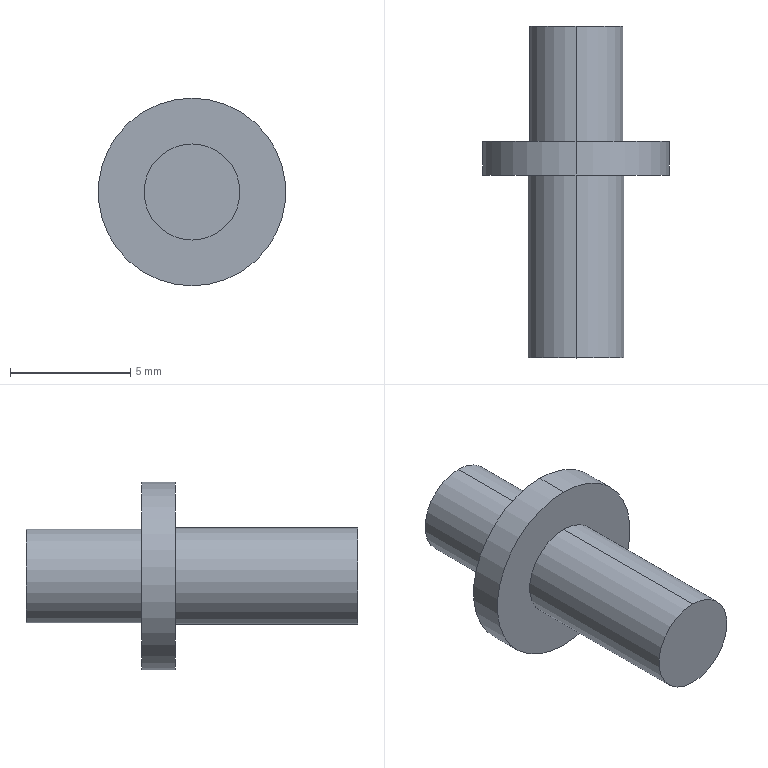Part | STEP file | Hinge lower door shaft 001 | 1 solid | 10 faces | box 7.8 x 13.8 x 7.8 mm | volume 219.742 mm3 | cylinder 6 | plane 4 | commonest cylinder face diameters 3.9 x2 4 x2 7.8 x2
STEP:
#1=CARTESIAN_POINT('',(0.,0.,0.));
#2=DIRECTION('',(0.,0.,1.));
#3=DIRECTION('',(1.,0.,0.));
#4=AXIS2_PLACEMENT_3D('',#1,#2,#3);
#5=CARTESIAN_POINT('',(0.,13.8,1.95));
#6=VERTEX_POINT('',#5);
#7=CARTESIAN_POINT('',(0.,13.8,-1.95));
#8=VERTEX_POINT('',#7);
#9=CARTESIAN_POINT('',(0.,13.8,0.));
#10=DIRECTION('',(0.,1.,0.));
#11=DIRECTION('',(0.,0.,1.));
#12=AXIS2_PLACEMENT_3D('',#9,#10,#11);
#13=CIRCLE('',#12,1.95);
#14=CARTESIAN_POINT('',(0.,13.8,0.));
#15=DIRECTION('',(0.,-1.,0.));
#16=DIRECTION('',(0.,0.,-1.));
#17=AXIS2_PLACEMENT_3D('',#14,#15,#16);
#18=CYLINDRICAL_SURFACE('',#17,1.95);
#19=CARTESIAN_POINT('',(3.142,0.));
#20=DIRECTION('',(-1.,0.));
#21=VECTOR('',#20,1.);
#22=LINE('',#19,#21);
#23=(GEOMETRIC_REPRESENTATION_CONTEXT(2)PARAMETRIC_REPRESENTATION_CONTEXT()REPRESENTATION_CONTEXT('',''));
#24=DEFINITIONAL_REPRESENTATION('',(#22),#23);
#25=PCURVE('',#18,#24);
#26=CARTESIAN_POINT('',(0.,13.8,0.));
#27=DIRECTION('',(0.,1.,0.));
#28=DIRECTION('',(1.,0.,0.));
#29=AXIS2_PLACEMENT_3D('',#26,#27,#28);
#30=PLANE('',#29);
#31=CARTESIAN_POINT('',(0.,0.));
#32=DIRECTION('',(0.,-1.));
#33=AXIS2_PLACEMENT_2D('',#31,#32);
#34=CIRCLE('',#33,1.95);
#35=(GEOMETRIC_REPRESENTATION_CONTEXT(2)PARAMETRIC_REPRESENTATION_CONTEXT()REPRESENTATION_CONTEXT('',''));
#36=DEFINITIONAL_REPRESENTATION('',(#34),#35);
#37=PCURVE('',#30,#36);
#38=SURFACE_CURVE('',#13,(#25,#37),.PCURVE_S1.);
#39=EDGE_CURVE('',#6,#8,#38,.T.);
#40=ORIENTED_EDGE('',*,*,#39,.F.);
#41=CARTESIAN_POINT('',(0.,9.,1.95));
#42=VERTEX_POINT('',#41);
#43=CARTESIAN_POINT('',(0.,13.8,1.95));
#44=DIRECTION('',(0.,-1.,0.));
#45=VECTOR('',#44,1.);
#46=LINE('',#43,#45);
#47=CARTESIAN_POINT('',(3.142,0.));
#48=DIRECTION('',(0.,1.));
#49=VECTOR('',#48,1.);
#50=LINE('',#47,#49);
#51=(GEOMETRIC_REPRESENTATION_CONTEXT(2)PARAMETRIC_REPRESENTATION_CONTEXT()REPRESENTATION_CONTEXT('',''));
#52=DEFINITIONAL_REPRESENTATION('',(#50),#51);
#53=PCURVE('',#18,#52);
#54=CARTESIAN_POINT('',(0.,13.8,0.));
#55=DIRECTION('',(0.,-1.,0.));
#56=DIRECTION('',(0.,0.,-1.));
#57=AXIS2_PLACEMENT_3D('',#54,#55,#56);
#58=CYLINDRICAL_SURFACE('',#57,1.95);
#59=CARTESIAN_POINT('',(3.142,0.));
#60=DIRECTION('',(0.,1.));
#61=VECTOR('',#60,1.);
#62=LINE('',#59,#61);
#63=(GEOMETRIC_REPRESENTATION_CONTEXT(2)PARAMETRIC_REPRESENTATION_CONTEXT()REPRESENTATION_CONTEXT('',''));
#64=DEFINITIONAL_REPRESENTATION('',(#62),#63);
#65=PCURVE('',#58,#64);
#66=SURFACE_CURVE('',#46,(#53,#65),.PCURVE_S1.);
#67=EDGE_CURVE('',#6,#42,#66,.T.);
#68=ORIENTED_EDGE('',*,*,#67,.T.);
#69=CARTESIAN_POINT('',(0.,9.,-1.95));
#70=VERTEX_POINT('',#69);
#71=CARTESIAN_POINT('',(0.,9.,0.));
#72=DIRECTION('',(0.,1.,0.));
#73=DIRECTION('',(0.,0.,1.));
#74=AXIS2_PLACEMENT_3D('',#71,#72,#73);
#75=CIRCLE('',#74,1.95);
#76=CARTESIAN_POINT('',(3.142,4.8));
#77=DIRECTION('',(-1.,0.));
#78=VECTOR('',#77,1.);
#79=LINE('',#76,#78);
#80=(GEOMETRIC_REPRESENTATION_CONTEXT(2)PARAMETRIC_REPRESENTATION_CONTEXT()REPRESENTATION_CONTEXT('',''));
#81=DEFINITIONAL_REPRESENTATION('',(#79),#80);
#82=PCURVE('',#18,#81);
#83=CARTESIAN_POINT('',(0.,9.,0.));
#84=DIRECTION('',(0.,1.,0.));
#85=DIRECTION('',(1.,0.,0.));
#86=AXIS2_PLACEMENT_3D('',#83,#84,#85);
#87=PLANE('',#86);
#88=CARTESIAN_POINT('',(0.,0.));
#89=DIRECTION('',(0.,-1.));
#90=AXIS2_PLACEMENT_2D('',#88,#89);
#91=CIRCLE('',#90,1.95);
#92=(GEOMETRIC_REPRESENTATION_CONTEXT(2)PARAMETRIC_REPRESENTATION_CONTEXT()REPRESENTATION_CONTEXT('',''));
#93=DEFINITIONAL_REPRESENTATION('',(#91),#92);
#94=PCURVE('',#87,#93);
#95=SURFACE_CURVE('',#75,(#82,#94),.PCURVE_S1.);
#96=EDGE_CURVE('',#42,#70,#95,.T.);
#97=ORIENTED_EDGE('',*,*,#96,.T.);
#98=CARTESIAN_POINT('',(0.,13.8,-1.95));
#99=DIRECTION('',(0.,-1.,0.));
#100=VECTOR('',#99,1.);
#101=LINE('',#98,#100);
#102=CARTESIAN_POINT('',(0.,0.));
#103=DIRECTION('',(0.,1.));
#104=VECTOR('',#103,1.);
#105=LINE('',#102,#104);
#106=(GEOMETRIC_REPRESENTATION_CONTEXT(2)PARAMETRIC_REPRESENTATION_CONTEXT()REPRESENTATION_CONTEXT('',''));
#107=DEFINITIONAL_REPRESENTATION('',(#105),#106);
#108=PCURVE('',#18,#107);
#109=CARTESIAN_POINT('',(6.283,0.));
#110=DIRECTION('',(0.,1.));
#111=VECTOR('',#110,1.);
#112=LINE('',#109,#111);
#113=(GEOMETRIC_REPRESENTATION_CONTEXT(2)PARAMETRIC_REPRESENTATION_CONTEXT()REPRESENTATION_CONTEXT('',''));
#114=DEFINITIONAL_REPRESENTATION('',(#112),#113);
#115=PCURVE('',#58,#114);
#116=SURFACE_CURVE('',#101,(#108,#115),.PCURVE_S1.);
#117=EDGE_CURVE('',#8,#70,#116,.T.);
#118=ORIENTED_EDGE('',*,*,#117,.F.);
#119=EDGE_LOOP('',(#40,#68,#97,#118));
#120=FACE_BOUND('',#119,.T.);
#121=ADVANCED_FACE('',(#120),#18,.T.);
#122=CARTESIAN_POINT('',(0.,9.,3.9));
#123=VERTEX_POINT('',#122);
#124=CARTESIAN_POINT('',(0.,9.,-3.9));
#125=VERTEX_POINT('',#124);
#126=CARTESIAN_POINT('',(0.,9.,0.));
#127=DIRECTION('',(0.,1.,0.));
#128=DIRECTION('',(0.,0.,1.));
#129=AXIS2_PLACEMENT_3D('',#126,#127,#128);
#130=CIRCLE('',#129,3.9);
#131=CARTESIAN_POINT('',(0.,9.,0.));
#132=DIRECTION('',(0.,-1.,0.));
#133=DIRECTION('',(0.,0.,-1.));
#134=AXIS2_PLACEMENT_3D('',#131,#132,#133);
#135=CYLINDRICAL_SURFACE('',#134,3.9);
#136=CARTESIAN_POINT('',(3.142,0.));
#137=DIRECTION('',(-1.,0.));
#138=VECTOR('',#137,1.);
#139=LINE('',#136,#138);
#140=(GEOMETRIC_REPRESENTATION_CONTEXT(2)PARAMETRIC_REPRESENTATION_CONTEXT()REPRESENTATION_CONTEXT('',''));
#141=DEFINITIONAL_REPRESENTATION('',(#139),#140);
#142=PCURVE('',#135,#141);
#143=CARTESIAN_POINT('',(0.,0.));
#144=DIRECTION('',(0.,-1.));
#145=AXIS2_PLACEMENT_2D('',#143,#144);
#146=CIRCLE('',#145,3.9);
#147=(GEOMETRIC_REPRESENTATION_CONTEXT(2)PARAMETRIC_REPRESENTATION_CONTEXT()REPRESENTATION_CONTEXT('',''));
#148=DEFINITIONAL_REPRESENTATION('',(#146),#147);
#149=PCURVE('',#87,#148);
#150=SURFACE_CURVE('',#130,(#142,#149),.PCURVE_S1.);
#151=EDGE_CURVE('',#123,#125,#150,.T.);
#152=ORIENTED_EDGE('',*,*,#151,.F.);
#153=CARTESIAN_POINT('',(0.,7.6,3.9));
#154=VERTEX_POINT('',#153);
#155=CARTESIAN_POINT('',(0.,9.,3.9));
#156=DIRECTION('',(0.,-1.,0.));
#157=VECTOR('',#156,1.);
#158=LINE('',#155,#157);
#159=CARTESIAN_POINT('',(3.142,0.));
#160=DIRECTION('',(0.,1.));
#161=VECTOR('',#160,1.);
#162=LINE('',#159,#161);
#163=(GEOMETRIC_REPRESENTATION_CONTEXT(2)PARAMETRIC_REPRESENTATION_CONTEXT()REPRESENTATION_CONTEXT('',''));
#164=DEFINITIONAL_REPRESENTATION('',(#162),#163);
#165=PCURVE('',#135,#164);
#166=CARTESIAN_POINT('',(0.,9.,0.));
#167=DIRECTION('',(0.,-1.,0.));
#168=DIRECTION('',(0.,0.,-1.));
#169=AXIS2_PLACEMENT_3D('',#166,#167,#168);
#170=CYLINDRICAL_SURFACE('',#169,3.9);
#171=CARTESIAN_POINT('',(3.142,0.));
#172=DIRECTION('',(0.,1.));
#173=VECTOR('',#172,1.);
#174=LINE('',#171,#173);
#175=(GEOMETRIC_REPRESENTATION_CONTEXT(2)PARAMETRIC_REPRESENTATION_CONTEXT()REPRESENTATION_CONTEXT('',''));
#176=DEFINITIONAL_REPRESENTATION('',(#174),#175);
#177=PCURVE('',#170,#176);
#178=SURFACE_CURVE('',#158,(#165,#177),.PCURVE_S1.);
#179=EDGE_CURVE('',#123,#154,#178,.T.);
#180=ORIENTED_EDGE('',*,*,#179,.T.);
#181=CARTESIAN_POINT('',(0.,7.6,-3.9));
#182=VERTEX_POINT('',#181);
#183=CARTESIAN_POINT('',(0.,7.6,0.));
#184=DIRECTION('',(0.,1.,0.));
#185=DIRECTION('',(0.,0.,1.));
#186=AXIS2_PLACEMENT_3D('',#183,#184,#185);
#187=CIRCLE('',#186,3.9);
#188=CARTESIAN_POINT('',(3.142,1.4));
#189=DIRECTION('',(-1.,0.));
#190=VECTOR('',#189,1.);
#191=LINE('',#188,#190);
#192=(GEOMETRIC_REPRESENTATION_CONTEXT(2)PARAMETRIC_REPRESENTATION_CONTEXT()REPRESENTATION_CONTEXT('',''));
#193=DEFINITIONAL_REPRESENTATION('',(#191),#192);
#194=PCURVE('',#135,#193);
#195=CARTESIAN_POINT('',(0.,7.6,0.));
#196=DIRECTION('',(0.,1.,0.));
#197=DIRECTION('',(1.,0.,0.));
#198=AXIS2_PLACEMENT_3D('',#195,#196,#197);
#199=PLANE('',#198);
#200=CARTESIAN_POINT('',(0.,0.));
#201=DIRECTION('',(0.,-1.));
#202=AXIS2_PLACEMENT_2D('',#200,#201);
#203=CIRCLE('',#202,3.9);
#204=(GEOMETRIC_REPRESENTATION_CONTEXT(2)PARAMETRIC_REPRESENTATION_CONTEXT()REPRESENTATION_CONTEXT('',''));
#205=DEFINITIONAL_REPRESENTATION('',(#203),#204);
#206=PCURVE('',#199,#205);
#207=SURFACE_CURVE('',#187,(#194,#206),.PCURVE_S1.);
#208=EDGE_CURVE('',#154,#182,#207,.T.);
#209=ORIENTED_EDGE('',*,*,#208,.T.);
#210=CARTESIAN_POINT('',(0.,9.,-3.9));
#211=DIRECTION('',(0.,-1.,0.));
#212=VECTOR('',#211,1.);
#213=LINE('',#210,#212);
#214=CARTESIAN_POINT('',(0.,0.));
#215=DIRECTION('',(0.,1.));
#216=VECTOR('',#215,1.);
#217=LINE('',#214,#216);
#218=(GEOMETRIC_REPRESENTATION_CONTEXT(2)PARAMETRIC_REPRESENTATION_CONTEXT()REPRESENTATION_CONTEXT('',''));
#219=DEFINITIONAL_REPRESENTATION('',(#217),#218);
#220=PCURVE('',#135,#219);
#221=CARTESIAN_POINT('',(6.283,0.));
#222=DIRECTION('',(0.,1.));
#223=VECTOR('',#222,1.);
#224=LINE('',#221,#223);
#225=(GEOMETRIC_REPRESENTATION_CONTEXT(2)PARAMETRIC_REPRESENTATION_CONTEXT()REPRESENTATION_CONTEXT('',''));
#226=DEFINITIONAL_REPRESENTATION('',(#224),#225);
#227=PCURVE('',#170,#226);
#228=SURFACE_CURVE('',#213,(#220,#227),.PCURVE_S1.);
#229=EDGE_CURVE('',#125,#182,#228,.T.);
#230=ORIENTED_EDGE('',*,*,#229,.F.);
#231=EDGE_LOOP('',(#152,#180,#209,#230));
#232=FACE_BOUND('',#231,.T.);
#233=ADVANCED_FACE('',(#232),#135,.T.);
#234=CARTESIAN_POINT('',(0.,7.6,2.));
#235=VERTEX_POINT('',#234);
#236=CARTESIAN_POINT('',(0.,7.6,-2.));
#237=VERTEX_POINT('',#236);
#238=CARTESIAN_POINT('',(0.,7.6,0.));
#239=DIRECTION('',(0.,1.,0.));
#240=DIRECTION('',(0.,0.,1.));
#241=AXIS2_PLACEMENT_3D('',#238,#239,#240);
#242=CIRCLE('',#241,2.);
#243=CARTESIAN_POINT('',(0.,7.6,0.));
#244=DIRECTION('',(0.,-1.,0.));
#245=DIRECTION('',(0.,0.,-1.));
#246=AXIS2_PLACEMENT_3D('',#243,#244,#245);
#247=CYLINDRICAL_SURFACE('',#246,2.);
#248=CARTESIAN_POINT('',(3.142,0.));
#249=DIRECTION('',(-1.,0.));
#250=VECTOR('',#249,1.);
#251=LINE('',#248,#250);
#252=(GEOMETRIC_REPRESENTATION_CONTEXT(2)PARAMETRIC_REPRESENTATION_CONTEXT()REPRESENTATION_CONTEXT('',''));
#253=DEFINITIONAL_REPRESENTATION('',(#251),#252);
#254=PCURVE('',#247,#253);
#255=CARTESIAN_POINT('',(0.,0.));
#256=DIRECTION('',(0.,-1.));
#257=AXIS2_PLACEMENT_2D('',#255,#256);
#258=CIRCLE('',#257,2.);
#259=(GEOMETRIC_REPRESENTATION_CONTEXT(2)PARAMETRIC_REPRESENTATION_CONTEXT()REPRESENTATION_CONTEXT('',''));
#260=DEFINITIONAL_REPRESENTATION('',(#258),#259);
#261=PCURVE('',#199,#260);
#262=SURFACE_CURVE('',#242,(#254,#261),.PCURVE_S1.);
#263=EDGE_CURVE('',#235,#237,#262,.T.);
#264=ORIENTED_EDGE('',*,*,#263,.F.);
#265=CARTESIAN_POINT('',(0.,0.,2.));
#266=VERTEX_POINT('',#265);
#267=CARTESIAN_POINT('',(0.,7.6,2.));
#268=DIRECTION('',(0.,-1.,0.));
#269=VECTOR('',#268,1.);
#270=LINE('',#267,#269);
#271=CARTESIAN_POINT('',(3.142,0.));
#272=DIRECTION('',(0.,1.));
#273=VECTOR('',#272,1.);
#274=LINE('',#271,#273);
#275=(GEOMETRIC_REPRESENTATION_CONTEXT(2)PARAMETRIC_REPRESENTATION_CONTEXT()REPRESENTATION_CONTEXT('',''));
#276=DEFINITIONAL_REPRESENTATION('',(#274),#275);
#277=PCURVE('',#247,#276);
#278=CARTESIAN_POINT('',(0.,7.6,0.));
#279=DIRECTION('',(0.,-1.,0.));
#280=DIRECTION('',(0.,0.,-1.));
#281=AXIS2_PLACEMENT_3D('',#278,#279,#280);
#282=CYLINDRICAL_SURFACE('',#281,2.);
#283=CARTESIAN_POINT('',(3.142,0.));
#284=DIRECTION('',(0.,1.));
#285=VECTOR('',#284,1.);
#286=LINE('',#283,#285);
#287=(GEOMETRIC_REPRESENTATION_CONTEXT(2)PARAMETRIC_REPRESENTATION_CONTEXT()REPRESENTATION_CONTEXT('',''));
#288=DEFINITIONAL_REPRESENTATION('',(#286),#287);
#289=PCURVE('',#282,#288);
#290=SURFACE_CURVE('',#270,(#277,#289),.PCURVE_S1.);
#291=EDGE_CURVE('',#235,#266,#290,.T.);
#292=ORIENTED_EDGE('',*,*,#291,.T.);
#293=CARTESIAN_POINT('',(0.,0.,-2.));
#294=VERTEX_POINT('',#293);
#295=CARTESIAN_POINT('',(0.,0.,0.));
#296=DIRECTION('',(0.,1.,0.));
#297=DIRECTION('',(0.,0.,1.));
#298=AXIS2_PLACEMENT_3D('',#295,#296,#297);
#299=CIRCLE('',#298,2.);
#300=CARTESIAN_POINT('',(3.142,7.6));
#301=DIRECTION('',(-1.,0.));
#302=VECTOR('',#301,1.);
#303=LINE('',#300,#302);
#304=(GEOMETRIC_REPRESENTATION_CONTEXT(2)PARAMETRIC_REPRESENTATION_CONTEXT()REPRESENTATION_CONTEXT('',''));
#305=DEFINITIONAL_REPRESENTATION('',(#303),#304);
#306=PCURVE('',#247,#305);
#307=CARTESIAN_POINT('',(0.,0.,0.));
#308=DIRECTION('',(0.,1.,0.));
#309=DIRECTION('',(1.,0.,0.));
#310=AXIS2_PLACEMENT_3D('',#307,#308,#309);
#311=PLANE('',#310);
#312=CARTESIAN_POINT('',(0.,0.));
#313=DIRECTION('',(0.,-1.));
#314=AXIS2_PLACEMENT_2D('',#312,#313);
#315=CIRCLE('',#314,2.);
#316=(GEOMETRIC_REPRESENTATION_CONTEXT(2)PARAMETRIC_REPRESENTATION_CONTEXT()REPRESENTATION_CONTEXT('',''));
#317=DEFINITIONAL_REPRESENTATION('',(#315),#316);
#318=PCURVE('',#311,#317);
#319=SURFACE_CURVE('',#299,(#306,#318),.PCURVE_S1.);
#320=EDGE_CURVE('',#266,#294,#319,.T.);
#321=ORIENTED_EDGE('',*,*,#320,.T.);
#322=CARTESIAN_POINT('',(0.,7.6,-2.));
#323=DIRECTION('',(0.,-1.,0.));
#324=VECTOR('',#323,1.);
#325=LINE('',#322,#324);
#326=CARTESIAN_POINT('',(0.,0.));
#327=DIRECTION('',(0.,1.));
#328=VECTOR('',#327,1.);
#329=LINE('',#326,#328);
#330=(GEOMETRIC_REPRESENTATION_CONTEXT(2)PARAMETRIC_REPRESENTATION_CONTEXT()REPRESENTATION_CONTEXT('',''));
#331=DEFINITIONAL_REPRESENTATION('',(#329),#330);
#332=PCURVE('',#247,#331);
#333=CARTESIAN_POINT('',(6.283,0.));
#334=DIRECTION('',(0.,1.));
#335=VECTOR('',#334,1.);
#336=LINE('',#333,#335);
#337=(GEOMETRIC_REPRESENTATION_CONTEXT(2)PARAMETRIC_REPRESENTATION_CONTEXT()REPRESENTATION_CONTEXT('',''));
#338=DEFINITIONAL_REPRESENTATION('',(#336),#337);
#339=PCURVE('',#282,#338);
#340=SURFACE_CURVE('',#325,(#332,#339),.PCURVE_S1.);
#341=EDGE_CURVE('',#237,#294,#340,.T.);
#342=ORIENTED_EDGE('',*,*,#341,.F.);
#343=EDGE_LOOP('',(#264,#292,#321,#342));
#344=FACE_BOUND('',#343,.T.);
#345=ADVANCED_FACE('',(#344),#247,.T.);
#346=CARTESIAN_POINT('',(0.,0.,0.));
#347=DIRECTION('',(0.,1.,0.));
#348=DIRECTION('',(0.,0.,1.));
#349=AXIS2_PLACEMENT_3D('',#346,#347,#348);
#350=CIRCLE('',#349,2.);
#351=CARTESIAN_POINT('',(0.,0.));
#352=DIRECTION('',(0.,-1.));
#353=AXIS2_PLACEMENT_2D('',#351,#352);
#354=CIRCLE('',#353,2.);
#355=(GEOMETRIC_REPRESENTATION_CONTEXT(2)PARAMETRIC_REPRESENTATION_CONTEXT()REPRESENTATION_CONTEXT('',''));
#356=DEFINITIONAL_REPRESENTATION('',(#354),#355);
#357=PCURVE('',#311,#356);
#358=CARTESIAN_POINT('',(9.425,7.6));
#359=DIRECTION('',(-1.,0.));
#360=VECTOR('',#359,1.);
#361=LINE('',#358,#360);
#362=(GEOMETRIC_REPRESENTATION_CONTEXT(2)PARAMETRIC_REPRESENTATION_CONTEXT()REPRESENTATION_CONTEXT('',''));
#363=DEFINITIONAL_REPRESENTATION('',(#361),#362);
#364=PCURVE('',#282,#363);
#365=SURFACE_CURVE('',#350,(#357,#364),.PCURVE_S1.);
#366=EDGE_CURVE('',#294,#266,#365,.T.);
#367=ORIENTED_EDGE('',*,*,#366,.F.);
#368=ORIENTED_EDGE('',*,*,#320,.F.);
#369=EDGE_LOOP('',(#367,#368));
#370=FACE_BOUND('',#369,.T.);
#371=ADVANCED_FACE('',(#370),#311,.F.);
#372=CARTESIAN_POINT('',(0.,9.,0.));
#373=DIRECTION('',(0.,1.,0.));
#374=DIRECTION('',(0.,0.,1.));
#375=AXIS2_PLACEMENT_3D('',#372,#373,#374);
#376=CIRCLE('',#375,1.95);
#377=CARTESIAN_POINT('',(0.,0.));
#378=DIRECTION('',(0.,-1.));
#379=AXIS2_PLACEMENT_2D('',#377,#378);
#380=CIRCLE('',#379,1.95);
#381=(GEOMETRIC_REPRESENTATION_CONTEXT(2)PARAMETRIC_REPRESENTATION_CONTEXT()REPRESENTATION_CONTEXT('',''));
#382=DEFINITIONAL_REPRESENTATION('',(#380),#381);
#383=PCURVE('',#87,#382);
#384=CARTESIAN_POINT('',(9.425,4.8));
#385=DIRECTION('',(-1.,0.));
#386=VECTOR('',#385,1.);
#387=LINE('',#384,#386);
#388=(GEOMETRIC_REPRESENTATION_CONTEXT(2)PARAMETRIC_REPRESENTATION_CONTEXT()REPRESENTATION_CONTEXT('',''));
#389=DEFINITIONAL_REPRESENTATION('',(#387),#388);
#390=PCURVE('',#58,#389);
#391=SURFACE_CURVE('',#376,(#383,#390),.PCURVE_S1.);
#392=EDGE_CURVE('',#70,#42,#391,.T.);
#393=ORIENTED_EDGE('',*,*,#392,.F.);
#394=ORIENTED_EDGE('',*,*,#96,.F.);
#395=EDGE_LOOP('',(#393,#394));
#396=FACE_BOUND('',#395,.T.);
#397=CARTESIAN_POINT('',(0.,9.,0.));
#398=DIRECTION('',(0.,1.,0.));
#399=DIRECTION('',(0.,0.,1.));
#400=AXIS2_PLACEMENT_3D('',#397,#398,#399);
#401=CIRCLE('',#400,3.9);
#402=CARTESIAN_POINT('',(0.,0.));
#403=DIRECTION('',(0.,-1.));
#404=AXIS2_PLACEMENT_2D('',#402,#403);
#405=CIRCLE('',#404,3.9);
#406=(GEOMETRIC_REPRESENTATION_CONTEXT(2)PARAMETRIC_REPRESENTATION_CONTEXT()REPRESENTATION_CONTEXT('',''));
#407=DEFINITIONAL_REPRESENTATION('',(#405),#406);
#408=PCURVE('',#87,#407);
#409=CARTESIAN_POINT('',(9.425,0.));
#410=DIRECTION('',(-1.,0.));
#411=VECTOR('',#410,1.);
#412=LINE('',#409,#411);
#413=(GEOMETRIC_REPRESENTATION_CONTEXT(2)PARAMETRIC_REPRESENTATION_CONTEXT()REPRESENTATION_CONTEXT('',''));
#414=DEFINITIONAL_REPRESENTATION('',(#412),#413);
#415=PCURVE('',#170,#414);
#416=SURFACE_CURVE('',#401,(#408,#415),.PCURVE_S1.);
#417=EDGE_CURVE('',#125,#123,#416,.T.);
#418=ORIENTED_EDGE('',*,*,#417,.T.);
#419=ORIENTED_EDGE('',*,*,#151,.T.);
#420=EDGE_LOOP('',(#418,#419));
#421=FACE_BOUND('',#420,.T.);
#422=ADVANCED_FACE('',(#396,#421),#87,.T.);
#423=CARTESIAN_POINT('',(0.,7.6,0.));
#424=DIRECTION('',(0.,1.,0.));
#425=DIRECTION('',(0.,0.,1.));
#426=AXIS2_PLACEMENT_3D('',#423,#424,#425);
#427=CIRCLE('',#426,2.);
#428=CARTESIAN_POINT('',(0.,0.));
#429=DIRECTION('',(0.,-1.));
#430=AXIS2_PLACEMENT_2D('',#428,#429);
#431=CIRCLE('',#430,2.);
#432=(GEOMETRIC_REPRESENTATION_CONTEXT(2)PARAMETRIC_REPRESENTATION_CONTEXT()REPRESENTATION_CONTEXT('',''));
#433=DEFINITIONAL_REPRESENTATION('',(#431),#432);
#434=PCURVE('',#199,#433);
#435=CARTESIAN_POINT('',(9.425,0.));
#436=DIRECTION('',(-1.,0.));
#437=VECTOR('',#436,1.);
#438=LINE('',#435,#437);
#439=(GEOMETRIC_REPRESENTATION_CONTEXT(2)PARAMETRIC_REPRESENTATION_CONTEXT()REPRESENTATION_CONTEXT('',''));
#440=DEFINITIONAL_REPRESENTATION('',(#438),#439);
#441=PCURVE('',#282,#440);
#442=SURFACE_CURVE('',#427,(#434,#441),.PCURVE_S1.);
#443=EDGE_CURVE('',#237,#235,#442,.T.);
#444=ORIENTED_EDGE('',*,*,#443,.T.);
#445=ORIENTED_EDGE('',*,*,#263,.T.);
#446=EDGE_LOOP('',(#444,#445));
#447=FACE_BOUND('',#446,.T.);
#448=CARTESIAN_POINT('',(0.,7.6,0.));
#449=DIRECTION('',(0.,1.,0.));
#450=DIRECTION('',(0.,0.,1.));
#451=AXIS2_PLACEMENT_3D('',#448,#449,#450);
#452=CIRCLE('',#451,3.9);
#453=CARTESIAN_POINT('',(0.,0.));
#454=DIRECTION('',(0.,-1.));
#455=AXIS2_PLACEMENT_2D('',#453,#454);
#456=CIRCLE('',#455,3.9);
#457=(GEOMETRIC_REPRESENTATION_CONTEXT(2)PARAMETRIC_REPRESENTATION_CONTEXT()REPRESENTATION_CONTEXT('',''));
#458=DEFINITIONAL_REPRESENTATION('',(#456),#457);
#459=PCURVE('',#199,#458);
#460=CARTESIAN_POINT('',(9.425,1.4));
#461=DIRECTION('',(-1.,0.));
#462=VECTOR('',#461,1.);
#463=LINE('',#460,#462);
#464=(GEOMETRIC_REPRESENTATION_CONTEXT(2)PARAMETRIC_REPRESENTATION_CONTEXT()REPRESENTATION_CONTEXT('',''));
#465=DEFINITIONAL_REPRESENTATION('',(#463),#464);
#466=PCURVE('',#170,#465);
#467=SURFACE_CURVE('',#452,(#459,#466),.PCURVE_S1.);
#468=EDGE_CURVE('',#182,#154,#467,.T.);
#469=ORIENTED_EDGE('',*,*,#468,.F.);
#470=ORIENTED_EDGE('',*,*,#208,.F.);
#471=EDGE_LOOP('',(#469,#470));
#472=FACE_BOUND('',#471,.T.);
#473=ADVANCED_FACE('',(#447,#472),#199,.F.);
#474=CARTESIAN_POINT('',(0.,13.8,0.));
#475=DIRECTION('',(0.,1.,0.));
#476=DIRECTION('',(0.,0.,1.));
#477=AXIS2_PLACEMENT_3D('',#474,#475,#476);
#478=CIRCLE('',#477,1.95);
#479=CARTESIAN_POINT('',(0.,0.));
#480=DIRECTION('',(0.,-1.));
#481=AXIS2_PLACEMENT_2D('',#479,#480);
#482=CIRCLE('',#481,1.95);
#483=(GEOMETRIC_REPRESENTATION_CONTEXT(2)PARAMETRIC_REPRESENTATION_CONTEXT()REPRESENTATION_CONTEXT('',''));
#484=DEFINITIONAL_REPRESENTATION('',(#482),#483);
#485=PCURVE('',#30,#484);
#486=CARTESIAN_POINT('',(9.425,0.));
#487=DIRECTION('',(-1.,0.));
#488=VECTOR('',#487,1.);
#489=LINE('',#486,#488);
#490=(GEOMETRIC_REPRESENTATION_CONTEXT(2)PARAMETRIC_REPRESENTATION_CONTEXT()REPRESENTATION_CONTEXT('',''));
#491=DEFINITIONAL_REPRESENTATION('',(#489),#490);
#492=PCURVE('',#58,#491);
#493=SURFACE_CURVE('',#478,(#485,#492),.PCURVE_S1.);
#494=EDGE_CURVE('',#8,#6,#493,.T.);
#495=ORIENTED_EDGE('',*,*,#494,.T.);
#496=ORIENTED_EDGE('',*,*,#39,.T.);
#497=EDGE_LOOP('',(#495,#496));
#498=FACE_BOUND('',#497,.T.);
#499=ADVANCED_FACE('',(#498),#30,.T.);
#500=ORIENTED_EDGE('',*,*,#291,.F.);
#501=ORIENTED_EDGE('',*,*,#443,.F.);
#502=ORIENTED_EDGE('',*,*,#341,.T.);
#503=ORIENTED_EDGE('',*,*,#366,.T.);
#504=EDGE_LOOP('',(#500,#501,#502,#503));
#505=FACE_BOUND('',#504,.T.);
#506=ADVANCED_FACE('',(#505),#282,.T.);
#507=ORIENTED_EDGE('',*,*,#179,.F.);
#508=ORIENTED_EDGE('',*,*,#417,.F.);
#509=ORIENTED_EDGE('',*,*,#229,.T.);
#510=ORIENTED_EDGE('',*,*,#468,.T.);
#511=EDGE_LOOP('',(#507,#508,#509,#510));
#512=FACE_BOUND('',#511,.T.);
#513=ADVANCED_FACE('',(#512),#170,.T.);
#514=ORIENTED_EDGE('',*,*,#67,.F.);
#515=ORIENTED_EDGE('',*,*,#494,.F.);
#516=ORIENTED_EDGE('',*,*,#117,.T.);
#517=ORIENTED_EDGE('',*,*,#392,.T.);
#518=EDGE_LOOP('',(#514,#515,#516,#517));
#519=FACE_BOUND('',#518,.T.);
#520=ADVANCED_FACE('',(#519),#58,.T.);
#521=CLOSED_SHELL('',(#121,#233,#345,#371,#422,#473,#499,#506,#513,#520));
#522=MANIFOLD_SOLID_BREP('',#521);
#523=(LENGTH_UNIT()NAMED_UNIT(*)SI_UNIT(.MILLI.,.METRE.));
#524=UNCERTAINTY_MEASURE_WITH_UNIT(LENGTH_MEASURE(0.0000001),#523,'','');
#525=(NAMED_UNIT(*)PLANE_ANGLE_UNIT()SI_UNIT($,.RADIAN.));
#526=(NAMED_UNIT(*)SI_UNIT($,.STERADIAN.)SOLID_ANGLE_UNIT());
#527=(GEOMETRIC_REPRESENTATION_CONTEXT(3)GLOBAL_UNCERTAINTY_ASSIGNED_CONTEXT((#524))GLOBAL_UNIT_ASSIGNED_CONTEXT((#523,#525,#526))REPRESENTATION_CONTEXT('',''));
#528=ADVANCED_BREP_SHAPE_REPRESENTATION('',(#4,#522),#527);